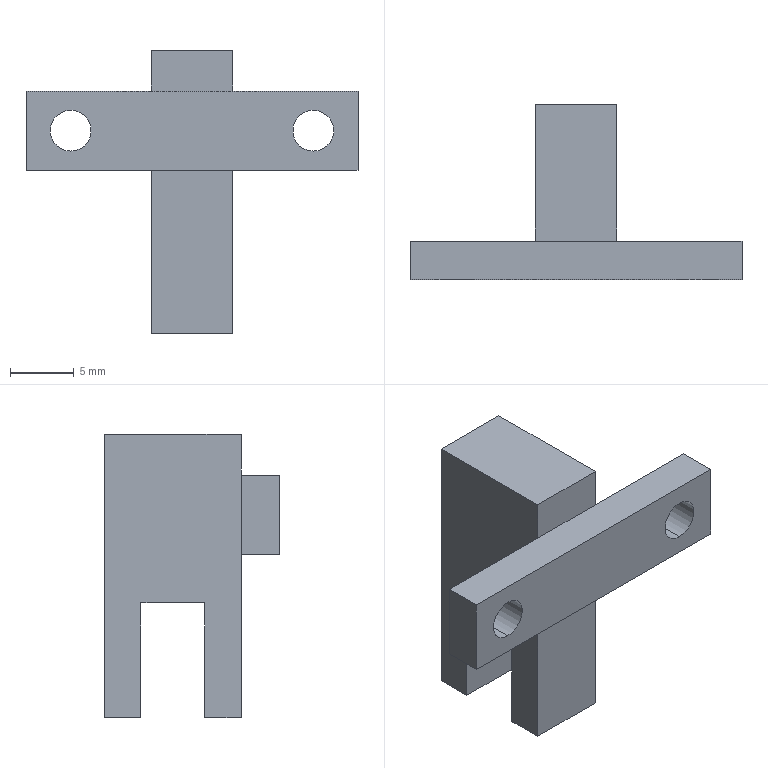Part | SolidWorks | features ICE 3, Extrusion 1 | 1 solid | 22 faces | box 26 x 13.7 x 22.2 mm | volume 1668 mm3 | plane 18 | cylinder 4 | commonest cylinder face diameters 3.2 x4
STEP:
#1=CARTESIAN_POINT('',(9.5,0.,-1.6));
#2=VERTEX_POINT('',#1);
#3=CARTESIAN_POINT('',(9.5,0.,1.6));
#4=VERTEX_POINT('',#3);
#5=CARTESIAN_POINT('',(9.5,0.,0.));
#6=DIRECTION('',(0.,1.,0.));
#7=DIRECTION('',(0.,0.,1.));
#8=AXIS2_PLACEMENT_3D('',#5,#6,#7);
#9=CIRCLE('',#8,1.6);
#10=EDGE_CURVE('',#2,#4,#9,.T.);
#11=ORIENTED_EDGE('',*,*,#10,.F.);
#12=CARTESIAN_POINT('',(9.5,3.,-1.6));
#13=VERTEX_POINT('',#12);
#14=CARTESIAN_POINT('',(9.5,-7.7,-1.6));
#15=DIRECTION('',(0.,1.,0.));
#16=VECTOR('',#15,1000.);
#17=LINE('',#14,#16);
#18=EDGE_CURVE('',#2,#13,#17,.T.);
#19=ORIENTED_EDGE('',*,*,#18,.T.);
#20=CARTESIAN_POINT('',(9.5,3.,1.6));
#21=VERTEX_POINT('',#20);
#22=CARTESIAN_POINT('',(9.5,3.,0.));
#23=DIRECTION('',(0.,1.,0.));
#24=DIRECTION('',(0.,0.,1.));
#25=AXIS2_PLACEMENT_3D('',#22,#23,#24);
#26=CIRCLE('',#25,1.6);
#27=EDGE_CURVE('',#13,#21,#26,.T.);
#28=ORIENTED_EDGE('',*,*,#27,.T.);
#29=CARTESIAN_POINT('',(9.5,-7.7,1.6));
#30=DIRECTION('',(0.,1.,0.));
#31=VECTOR('',#30,1000.);
#32=LINE('',#29,#31);
#33=EDGE_CURVE('',#4,#21,#32,.T.);
#34=ORIENTED_EDGE('',*,*,#33,.F.);
#35=EDGE_LOOP('',(#11,#19,#28,#34));
#36=FACE_OUTER_BOUND('',#35,.T.);
#37=CARTESIAN_POINT('',(9.5,-7.7,0.));
#38=DIRECTION('',(0.,1.,0.));
#39=DIRECTION('',(0.,0.,1.));
#40=AXIS2_PLACEMENT_3D('',#37,#38,#39);
#41=CYLINDRICAL_SURFACE('',#40,1.6);
#42=ADVANCED_FACE('',(#36),#41,.F.);
#43=CARTESIAN_POINT('',(-9.5,0.,-1.6));
#44=VERTEX_POINT('',#43);
#45=CARTESIAN_POINT('',(-9.5,0.,1.6));
#46=VERTEX_POINT('',#45);
#47=CARTESIAN_POINT('',(-9.5,0.,0.));
#48=DIRECTION('',(0.,1.,0.));
#49=DIRECTION('',(0.,0.,1.));
#50=AXIS2_PLACEMENT_3D('',#47,#48,#49);
#51=CIRCLE('',#50,1.6);
#52=EDGE_CURVE('',#44,#46,#51,.T.);
#53=ORIENTED_EDGE('',*,*,#52,.F.);
#54=CARTESIAN_POINT('',(-9.5,3.,-1.6));
#55=VERTEX_POINT('',#54);
#56=CARTESIAN_POINT('',(-9.5,-7.7,-1.6));
#57=DIRECTION('',(0.,1.,0.));
#58=VECTOR('',#57,1000.);
#59=LINE('',#56,#58);
#60=EDGE_CURVE('',#44,#55,#59,.T.);
#61=ORIENTED_EDGE('',*,*,#60,.T.);
#62=CARTESIAN_POINT('',(-9.5,3.,1.6));
#63=VERTEX_POINT('',#62);
#64=CARTESIAN_POINT('',(-9.5,3.,0.));
#65=DIRECTION('',(0.,1.,0.));
#66=DIRECTION('',(0.,0.,1.));
#67=AXIS2_PLACEMENT_3D('',#64,#65,#66);
#68=CIRCLE('',#67,1.6);
#69=EDGE_CURVE('',#55,#63,#68,.T.);
#70=ORIENTED_EDGE('',*,*,#69,.T.);
#71=CARTESIAN_POINT('',(-9.5,-7.7,1.6));
#72=DIRECTION('',(0.,1.,0.));
#73=VECTOR('',#72,1000.);
#74=LINE('',#71,#73);
#75=EDGE_CURVE('',#46,#63,#74,.T.);
#76=ORIENTED_EDGE('',*,*,#75,.F.);
#77=EDGE_LOOP('',(#53,#61,#70,#76));
#78=FACE_OUTER_BOUND('',#77,.T.);
#79=CARTESIAN_POINT('',(-9.5,-7.7,0.));
#80=DIRECTION('',(0.,1.,0.));
#81=DIRECTION('',(0.,0.,1.));
#82=AXIS2_PLACEMENT_3D('',#79,#80,#81);
#83=CYLINDRICAL_SURFACE('',#82,1.6);
#84=ADVANCED_FACE('',(#78),#83,.F.);
#85=CARTESIAN_POINT('',(3.2,13.7,-15.9));
#86=VERTEX_POINT('',#85);
#87=CARTESIAN_POINT('',(3.2,10.85,-15.9));
#88=VERTEX_POINT('',#87);
#89=CARTESIAN_POINT('',(3.2,13.7,-15.9));
#90=DIRECTION('',(0.,-1.,0.));
#91=VECTOR('',#90,1000.);
#92=LINE('',#89,#91);
#93=EDGE_CURVE('',#86,#88,#92,.T.);
#94=ORIENTED_EDGE('',*,*,#93,.T.);
#95=CARTESIAN_POINT('',(-3.2,10.85,-15.9));
#96=VERTEX_POINT('',#95);
#97=CARTESIAN_POINT('',(-3.2,10.85,-15.9));
#98=DIRECTION('',(-1.,0.,0.));
#99=VECTOR('',#98,1000.);
#100=LINE('',#97,#99);
#101=EDGE_CURVE('',#88,#96,#100,.T.);
#102=ORIENTED_EDGE('',*,*,#101,.T.);
#103=CARTESIAN_POINT('',(-3.2,13.7,-15.9));
#104=VERTEX_POINT('',#103);
#105=CARTESIAN_POINT('',(-3.2,13.7,-15.9));
#106=DIRECTION('',(0.,-1.,0.));
#107=VECTOR('',#106,1000.);
#108=LINE('',#105,#107);
#109=EDGE_CURVE('',#104,#96,#108,.T.);
#110=ORIENTED_EDGE('',*,*,#109,.F.);
#111=CARTESIAN_POINT('',(-3.2,13.7,-15.9));
#112=DIRECTION('',(-1.,0.,0.));
#113=VECTOR('',#112,1000.);
#114=LINE('',#111,#113);
#115=EDGE_CURVE('',#86,#104,#114,.T.);
#116=ORIENTED_EDGE('',*,*,#115,.F.);
#117=EDGE_LOOP('',(#94,#102,#110,#116));
#118=FACE_OUTER_BOUND('',#117,.T.);
#119=CARTESIAN_POINT('',(-3.2,13.7,-15.9));
#120=DIRECTION('',(0.,0.,1.));
#121=DIRECTION('',(1.,0.,0.));
#122=AXIS2_PLACEMENT_3D('',#119,#120,#121);
#123=PLANE('',#122);
#124=ADVANCED_FACE('',(#118),#123,.F.);
#125=CARTESIAN_POINT('',(-9.5,3.,0.));
#126=DIRECTION('',(0.,1.,0.));
#127=DIRECTION('',(0.,0.,1.));
#128=AXIS2_PLACEMENT_3D('',#125,#126,#127);
#129=CIRCLE('',#128,1.6);
#130=EDGE_CURVE('',#63,#55,#129,.T.);
#131=ORIENTED_EDGE('',*,*,#130,.F.);
#132=ORIENTED_EDGE('',*,*,#69,.F.);
#133=EDGE_LOOP('',(#131,#132));
#134=FACE_BOUND('',#133,.T.);
#135=CARTESIAN_POINT('',(-3.2,3.,-3.1));
#136=VERTEX_POINT('',#135);
#137=CARTESIAN_POINT('',(-3.2,3.,3.1));
#138=VERTEX_POINT('',#137);
#139=CARTESIAN_POINT('',(-3.2,3.,-15.9));
#140=DIRECTION('',(0.,0.,1.));
#141=VECTOR('',#140,1000.);
#142=LINE('',#139,#141);
#143=EDGE_CURVE('',#136,#138,#142,.T.);
#144=ORIENTED_EDGE('',*,*,#143,.F.);
#145=CARTESIAN_POINT('',(-13.,3.,-3.1));
#146=VERTEX_POINT('',#145);
#147=CARTESIAN_POINT('',(-13.,3.,-3.1));
#148=DIRECTION('',(-1.,0.,0.));
#149=VECTOR('',#148,1000.);
#150=LINE('',#147,#149);
#151=EDGE_CURVE('',#136,#146,#150,.T.);
#152=ORIENTED_EDGE('',*,*,#151,.T.);
#153=CARTESIAN_POINT('',(-13.,3.,3.1));
#154=VERTEX_POINT('',#153);
#155=CARTESIAN_POINT('',(-13.,3.,-3.1));
#156=DIRECTION('',(0.,0.,1.));
#157=VECTOR('',#156,1000.);
#158=LINE('',#155,#157);
#159=EDGE_CURVE('',#146,#154,#158,.T.);
#160=ORIENTED_EDGE('',*,*,#159,.T.);
#161=CARTESIAN_POINT('',(-13.,3.,3.1));
#162=DIRECTION('',(1.,0.,0.));
#163=VECTOR('',#162,1000.);
#164=LINE('',#161,#163);
#165=EDGE_CURVE('',#154,#138,#164,.T.);
#166=ORIENTED_EDGE('',*,*,#165,.T.);
#167=EDGE_LOOP('',(#144,#152,#160,#166));
#168=FACE_OUTER_BOUND('',#167,.T.);
#169=CARTESIAN_POINT('',(0.,3.,0.));
#170=DIRECTION('',(0.,1.,0.));
#171=DIRECTION('',(0.,0.,1.));
#172=AXIS2_PLACEMENT_3D('',#169,#170,#171);
#173=PLANE('',#172);
#174=ADVANCED_FACE('',(#134,#168),#173,.T.);
#175=CARTESIAN_POINT('',(13.,0.,3.1));
#176=VERTEX_POINT('',#175);
#177=CARTESIAN_POINT('',(13.,0.,-3.1));
#178=VERTEX_POINT('',#177);
#179=CARTESIAN_POINT('',(13.,0.,-3.1));
#180=DIRECTION('',(0.,0.,-1.));
#181=VECTOR('',#180,1000.);
#182=LINE('',#179,#181);
#183=EDGE_CURVE('',#176,#178,#182,.T.);
#184=ORIENTED_EDGE('',*,*,#183,.T.);
#185=CARTESIAN_POINT('',(13.,3.,-3.1));
#186=VERTEX_POINT('',#185);
#187=CARTESIAN_POINT('',(13.,3.,-3.1));
#188=DIRECTION('',(0.,-1.,0.));
#189=VECTOR('',#188,1000.);
#190=LINE('',#187,#189);
#191=EDGE_CURVE('',#186,#178,#190,.T.);
#192=ORIENTED_EDGE('',*,*,#191,.F.);
#193=CARTESIAN_POINT('',(13.,3.,3.1));
#194=VERTEX_POINT('',#193);
#195=CARTESIAN_POINT('',(13.,3.,-3.1));
#196=DIRECTION('',(0.,0.,-1.));
#197=VECTOR('',#196,1000.);
#198=LINE('',#195,#197);
#199=EDGE_CURVE('',#194,#186,#198,.T.);
#200=ORIENTED_EDGE('',*,*,#199,.F.);
#201=CARTESIAN_POINT('',(13.,3.,3.1));
#202=DIRECTION('',(0.,-1.,0.));
#203=VECTOR('',#202,1000.);
#204=LINE('',#201,#203);
#205=EDGE_CURVE('',#194,#176,#204,.T.);
#206=ORIENTED_EDGE('',*,*,#205,.T.);
#207=EDGE_LOOP('',(#184,#192,#200,#206));
#208=FACE_OUTER_BOUND('',#207,.T.);
#209=CARTESIAN_POINT('',(13.,3.,-3.1));
#210=DIRECTION('',(-1.,0.,0.));
#211=DIRECTION('',(0.,0.,1.));
#212=AXIS2_PLACEMENT_3D('',#209,#210,#211);
#213=PLANE('',#212);
#214=ADVANCED_FACE('',(#208),#213,.F.);
#215=CARTESIAN_POINT('',(-13.,0.,-3.1));
#216=VERTEX_POINT('',#215);
#217=CARTESIAN_POINT('',(-13.,0.,-3.1));
#218=DIRECTION('',(-1.,0.,0.));
#219=VECTOR('',#218,1000.);
#220=LINE('',#217,#219);
#221=EDGE_CURVE('',#178,#216,#220,.T.);
#222=ORIENTED_EDGE('',*,*,#221,.T.);
#223=CARTESIAN_POINT('',(-13.,3.,-3.1));
#224=DIRECTION('',(0.,-1.,0.));
#225=VECTOR('',#224,1000.);
#226=LINE('',#223,#225);
#227=EDGE_CURVE('',#146,#216,#226,.T.);
#228=ORIENTED_EDGE('',*,*,#227,.F.);
#229=ORIENTED_EDGE('',*,*,#151,.F.);
#230=CARTESIAN_POINT('',(3.2,3.,-3.1));
#231=VERTEX_POINT('',#230);
#232=CARTESIAN_POINT('',(-13.,3.,-3.1));
#233=DIRECTION('',(-1.,0.,0.));
#234=VECTOR('',#233,1000.);
#235=LINE('',#232,#234);
#236=EDGE_CURVE('',#231,#136,#235,.T.);
#237=ORIENTED_EDGE('',*,*,#236,.F.);
#238=CARTESIAN_POINT('',(-13.,3.,-3.1));
#239=DIRECTION('',(-1.,0.,0.));
#240=VECTOR('',#239,1000.);
#241=LINE('',#238,#240);
#242=EDGE_CURVE('',#186,#231,#241,.T.);
#243=ORIENTED_EDGE('',*,*,#242,.F.);
#244=ORIENTED_EDGE('',*,*,#191,.T.);
#245=EDGE_LOOP('',(#222,#228,#229,#237,#243,#244));
#246=FACE_OUTER_BOUND('',#245,.T.);
#247=CARTESIAN_POINT('',(-13.,3.,-3.1));
#248=DIRECTION('',(0.,0.,1.));
#249=DIRECTION('',(1.,0.,0.));
#250=AXIS2_PLACEMENT_3D('',#247,#248,#249);
#251=PLANE('',#250);
#252=ADVANCED_FACE('',(#246),#251,.F.);
#253=CARTESIAN_POINT('',(-13.,0.,3.1));
#254=VERTEX_POINT('',#253);
#255=CARTESIAN_POINT('',(-13.,0.,-3.1));
#256=DIRECTION('',(0.,0.,1.));
#257=VECTOR('',#256,1000.);
#258=LINE('',#255,#257);
#259=EDGE_CURVE('',#216,#254,#258,.T.);
#260=ORIENTED_EDGE('',*,*,#259,.T.);
#261=CARTESIAN_POINT('',(-13.,3.,3.1));
#262=DIRECTION('',(0.,-1.,0.));
#263=VECTOR('',#262,1000.);
#264=LINE('',#261,#263);
#265=EDGE_CURVE('',#154,#254,#264,.T.);
#266=ORIENTED_EDGE('',*,*,#265,.F.);
#267=ORIENTED_EDGE('',*,*,#159,.F.);
#268=ORIENTED_EDGE('',*,*,#227,.T.);
#269=EDGE_LOOP('',(#260,#266,#267,#268));
#270=FACE_OUTER_BOUND('',#269,.T.);
#271=CARTESIAN_POINT('',(-13.,3.,-3.1));
#272=DIRECTION('',(1.,0.,0.));
#273=DIRECTION('',(0.,0.,-1.));
#274=AXIS2_PLACEMENT_3D('',#271,#272,#273);
#275=PLANE('',#274);
#276=ADVANCED_FACE('',(#270),#275,.F.);
#277=CARTESIAN_POINT('',(-13.,0.,3.1));
#278=DIRECTION('',(1.,0.,0.));
#279=VECTOR('',#278,1000.);
#280=LINE('',#277,#279);
#281=EDGE_CURVE('',#254,#176,#280,.T.);
#282=ORIENTED_EDGE('',*,*,#281,.T.);
#283=ORIENTED_EDGE('',*,*,#205,.F.);
#284=CARTESIAN_POINT('',(3.2,3.,3.1));
#285=VERTEX_POINT('',#284);
#286=CARTESIAN_POINT('',(-13.,3.,3.1));
#287=DIRECTION('',(1.,0.,0.));
#288=VECTOR('',#287,1000.);
#289=LINE('',#286,#288);
#290=EDGE_CURVE('',#285,#194,#289,.T.);
#291=ORIENTED_EDGE('',*,*,#290,.F.);
#292=CARTESIAN_POINT('',(-13.,3.,3.1));
#293=DIRECTION('',(1.,0.,0.));
#294=VECTOR('',#293,1000.);
#295=LINE('',#292,#294);
#296=EDGE_CURVE('',#138,#285,#295,.T.);
#297=ORIENTED_EDGE('',*,*,#296,.F.);
#298=ORIENTED_EDGE('',*,*,#165,.F.);
#299=ORIENTED_EDGE('',*,*,#265,.T.);
#300=EDGE_LOOP('',(#282,#283,#291,#297,#298,#299));
#301=FACE_OUTER_BOUND('',#300,.T.);
#302=CARTESIAN_POINT('',(-13.,3.,3.1));
#303=DIRECTION('',(0.,0.,-1.));
#304=DIRECTION('',(-1.,0.,0.));
#305=AXIS2_PLACEMENT_3D('',#302,#303,#304);
#306=PLANE('',#305);
#307=ADVANCED_FACE('',(#301),#306,.F.);
#308=CARTESIAN_POINT('',(9.5,3.,0.));
#309=DIRECTION('',(0.,1.,0.));
#310=DIRECTION('',(0.,0.,1.));
#311=AXIS2_PLACEMENT_3D('',#308,#309,#310);
#312=CIRCLE('',#311,1.6);
#313=EDGE_CURVE('',#21,#13,#312,.T.);
#314=ORIENTED_EDGE('',*,*,#313,.F.);
#315=ORIENTED_EDGE('',*,*,#27,.F.);
#316=EDGE_LOOP('',(#314,#315));
#317=FACE_BOUND('',#316,.T.);
#318=CARTESIAN_POINT('',(3.2,3.,-15.9));
#319=DIRECTION('',(0.,0.,-1.));
#320=VECTOR('',#319,1000.);
#321=LINE('',#318,#320);
#322=EDGE_CURVE('',#285,#231,#321,.T.);
#323=ORIENTED_EDGE('',*,*,#322,.F.);
#324=ORIENTED_EDGE('',*,*,#290,.T.);
#325=ORIENTED_EDGE('',*,*,#199,.T.);
#326=ORIENTED_EDGE('',*,*,#242,.T.);
#327=EDGE_LOOP('',(#323,#324,#325,#326));
#328=FACE_OUTER_BOUND('',#327,.T.);
#329=CARTESIAN_POINT('',(0.,3.,0.));
#330=DIRECTION('',(0.,1.,0.));
#331=DIRECTION('',(0.,0.,1.));
#332=AXIS2_PLACEMENT_3D('',#329,#330,#331);
#333=PLANE('',#332);
#334=ADVANCED_FACE('',(#317,#328),#333,.T.);
#335=CARTESIAN_POINT('',(9.5,0.,0.));
#336=DIRECTION('',(0.,1.,0.));
#337=DIRECTION('',(0.,0.,1.));
#338=AXIS2_PLACEMENT_3D('',#335,#336,#337);
#339=CIRCLE('',#338,1.6);
#340=EDGE_CURVE('',#4,#2,#339,.T.);
#341=ORIENTED_EDGE('',*,*,#340,.T.);
#342=ORIENTED_EDGE('',*,*,#10,.T.);
#343=EDGE_LOOP('',(#341,#342));
#344=FACE_BOUND('',#343,.T.);
#345=CARTESIAN_POINT('',(-9.5,0.,0.));
#346=DIRECTION('',(0.,1.,0.));
#347=DIRECTION('',(0.,0.,1.));
#348=AXIS2_PLACEMENT_3D('',#345,#346,#347);
#349=CIRCLE('',#348,1.6);
#350=EDGE_CURVE('',#46,#44,#349,.T.);
#351=ORIENTED_EDGE('',*,*,#350,.T.);
#352=ORIENTED_EDGE('',*,*,#52,.T.);
#353=EDGE_LOOP('',(#351,#352));
#354=FACE_BOUND('',#353,.T.);
#355=ORIENTED_EDGE('',*,*,#183,.F.);
#356=ORIENTED_EDGE('',*,*,#281,.F.);
#357=ORIENTED_EDGE('',*,*,#259,.F.);
#358=ORIENTED_EDGE('',*,*,#221,.F.);
#359=EDGE_LOOP('',(#355,#356,#357,#358));
#360=FACE_OUTER_BOUND('',#359,.T.);
#361=CARTESIAN_POINT('',(0.,0.,0.));
#362=DIRECTION('',(0.,1.,0.));
#363=DIRECTION('',(0.,0.,1.));
#364=AXIS2_PLACEMENT_3D('',#361,#362,#363);
#365=PLANE('',#364);
#366=ADVANCED_FACE('',(#344,#354,#360),#365,.F.);
#367=CARTESIAN_POINT('',(3.2,3.,-15.9));
#368=VERTEX_POINT('',#367);
#369=CARTESIAN_POINT('',(3.2,3.,-15.9));
#370=DIRECTION('',(0.,0.,-1.));
#371=VECTOR('',#370,1000.);
#372=LINE('',#369,#371);
#373=EDGE_CURVE('',#231,#368,#372,.T.);
#374=ORIENTED_EDGE('',*,*,#373,.F.);
#375=ORIENTED_EDGE('',*,*,#236,.T.);
#376=CARTESIAN_POINT('',(-3.2,3.,-15.9));
#377=VERTEX_POINT('',#376);
#378=CARTESIAN_POINT('',(-3.2,3.,-15.9));
#379=DIRECTION('',(0.,0.,1.));
#380=VECTOR('',#379,1000.);
#381=LINE('',#378,#380);
#382=EDGE_CURVE('',#377,#136,#381,.T.);
#383=ORIENTED_EDGE('',*,*,#382,.F.);
#384=CARTESIAN_POINT('',(-3.2,3.,-15.9));
#385=DIRECTION('',(-1.,0.,0.));
#386=VECTOR('',#385,1000.);
#387=LINE('',#384,#386);
#388=EDGE_CURVE('',#368,#377,#387,.T.);
#389=ORIENTED_EDGE('',*,*,#388,.F.);
#390=EDGE_LOOP('',(#374,#375,#383,#389));
#391=FACE_OUTER_BOUND('',#390,.T.);
#392=CARTESIAN_POINT('',(0.,3.,0.));
#393=DIRECTION('',(0.,1.,0.));
#394=DIRECTION('',(0.,0.,1.));
#395=AXIS2_PLACEMENT_3D('',#392,#393,#394);
#396=PLANE('',#395);
#397=ADVANCED_FACE('',(#391),#396,.F.);
#398=CARTESIAN_POINT('',(-3.2,3.,6.3));
#399=VERTEX_POINT('',#398);
#400=CARTESIAN_POINT('',(-3.2,3.,-15.9));
#401=DIRECTION('',(0.,0.,1.));
#402=VECTOR('',#401,1000.);
#403=LINE('',#400,#402);
#404=EDGE_CURVE('',#138,#399,#403,.T.);
#405=ORIENTED_EDGE('',*,*,#404,.F.);
#406=ORIENTED_EDGE('',*,*,#296,.T.);
#407=CARTESIAN_POINT('',(3.2,3.,6.3));
#408=VERTEX_POINT('',#407);
#409=CARTESIAN_POINT('',(3.2,3.,-15.9));
#410=DIRECTION('',(0.,0.,-1.));
#411=VECTOR('',#410,1000.);
#412=LINE('',#409,#411);
#413=EDGE_CURVE('',#408,#285,#412,.T.);
#414=ORIENTED_EDGE('',*,*,#413,.F.);
#415=CARTESIAN_POINT('',(-3.2,3.,6.3));
#416=DIRECTION('',(1.,0.,0.));
#417=VECTOR('',#416,1000.);
#418=LINE('',#415,#417);
#419=EDGE_CURVE('',#399,#408,#418,.T.);
#420=ORIENTED_EDGE('',*,*,#419,.F.);
#421=EDGE_LOOP('',(#405,#406,#414,#420));
#422=FACE_OUTER_BOUND('',#421,.T.);
#423=CARTESIAN_POINT('',(0.,3.,0.));
#424=DIRECTION('',(0.,1.,0.));
#425=DIRECTION('',(0.,0.,1.));
#426=AXIS2_PLACEMENT_3D('',#423,#424,#425);
#427=PLANE('',#426);
#428=ADVANCED_FACE('',(#422),#427,.F.);
#429=ORIENTED_EDGE('',*,*,#109,.T.);
#430=CARTESIAN_POINT('',(-3.2,10.85,-6.9));
#431=VERTEX_POINT('',#430);
#432=CARTESIAN_POINT('',(-3.2,10.85,-15.9));
#433=DIRECTION('',(0.,0.,-1.));
#434=VECTOR('',#433,1000.);
#435=LINE('',#432,#434);
#436=EDGE_CURVE('',#431,#96,#435,.T.);
#437=ORIENTED_EDGE('',*,*,#436,.F.);
#438=CARTESIAN_POINT('',(-3.2,5.85,-6.9));
#439=VERTEX_POINT('',#438);
#440=CARTESIAN_POINT('',(-3.2,10.85,-6.9));
#441=DIRECTION('',(0.,1.,0.));
#442=VECTOR('',#441,1000.);
#443=LINE('',#440,#442);
#444=EDGE_CURVE('',#439,#431,#443,.T.);
#445=ORIENTED_EDGE('',*,*,#444,.F.);
#446=CARTESIAN_POINT('',(-3.2,5.85,-15.9));
#447=VERTEX_POINT('',#446);
#448=CARTESIAN_POINT('',(-3.2,5.85,-15.9));
#449=DIRECTION('',(0.,0.,1.));
#450=VECTOR('',#449,1000.);
#451=LINE('',#448,#450);
#452=EDGE_CURVE('',#447,#439,#451,.T.);
#453=ORIENTED_EDGE('',*,*,#452,.F.);
#454=CARTESIAN_POINT('',(-3.2,13.7,-15.9));
#455=DIRECTION('',(0.,-1.,0.));
#456=VECTOR('',#455,1000.);
#457=LINE('',#454,#456);
#458=EDGE_CURVE('',#447,#377,#457,.T.);
#459=ORIENTED_EDGE('',*,*,#458,.T.);
#460=ORIENTED_EDGE('',*,*,#382,.T.);
#461=ORIENTED_EDGE('',*,*,#143,.T.);
#462=ORIENTED_EDGE('',*,*,#404,.T.);
#463=CARTESIAN_POINT('',(-3.2,13.7,6.3));
#464=VERTEX_POINT('',#463);
#465=CARTESIAN_POINT('',(-3.2,13.7,6.3));
#466=DIRECTION('',(0.,-1.,0.));
#467=VECTOR('',#466,1000.);
#468=LINE('',#465,#467);
#469=EDGE_CURVE('',#464,#399,#468,.T.);
#470=ORIENTED_EDGE('',*,*,#469,.F.);
#471=CARTESIAN_POINT('',(-3.2,13.7,-15.9));
#472=DIRECTION('',(0.,0.,1.));
#473=VECTOR('',#472,1000.);
#474=LINE('',#471,#473);
#475=EDGE_CURVE('',#104,#464,#474,.T.);
#476=ORIENTED_EDGE('',*,*,#475,.F.);
#477=EDGE_LOOP('',(#429,#437,#445,#453,#459,#460,#461,#462,#470,#476));
#478=FACE_OUTER_BOUND('',#477,.T.);
#479=CARTESIAN_POINT('',(-3.2,13.7,-15.9));
#480=DIRECTION('',(1.,0.,0.));
#481=DIRECTION('',(0.,0.,-1.));
#482=AXIS2_PLACEMENT_3D('',#479,#480,#481);
#483=PLANE('',#482);
#484=ADVANCED_FACE('',(#478),#483,.F.);
#485=ORIENTED_EDGE('',*,*,#419,.T.);
#486=CARTESIAN_POINT('',(3.2,13.7,6.3));
#487=VERTEX_POINT('',#486);
#488=CARTESIAN_POINT('',(3.2,13.7,6.3));
#489=DIRECTION('',(0.,-1.,0.));
#490=VECTOR('',#489,1000.);
#491=LINE('',#488,#490);
#492=EDGE_CURVE('',#487,#408,#491,.T.);
#493=ORIENTED_EDGE('',*,*,#492,.F.);
#494=CARTESIAN_POINT('',(-3.2,13.7,6.3));
#495=DIRECTION('',(1.,0.,0.));
#496=VECTOR('',#495,1000.);
#497=LINE('',#494,#496);
#498=EDGE_CURVE('',#464,#487,#497,.T.);
#499=ORIENTED_EDGE('',*,*,#498,.F.);
#500=ORIENTED_EDGE('',*,*,#469,.T.);
#501=EDGE_LOOP('',(#485,#493,#499,#500));
#502=FACE_OUTER_BOUND('',#501,.T.);
#503=CARTESIAN_POINT('',(-3.2,13.7,6.3));
#504=DIRECTION('',(0.,0.,-1.));
#505=DIRECTION('',(-1.,0.,0.));
#506=AXIS2_PLACEMENT_3D('',#503,#504,#505);
#507=PLANE('',#506);
#508=ADVANCED_FACE('',(#502),#507,.F.);
#509=CARTESIAN_POINT('',(3.2,5.85,-6.9));
#510=VERTEX_POINT('',#509);
#511=CARTESIAN_POINT('',(3.2,10.85,-6.9));
#512=VERTEX_POINT('',#511);
#513=CARTESIAN_POINT('',(3.2,13.7,-6.9));
#514=DIRECTION('',(0.,1.,0.));
#515=VECTOR('',#514,1000.);
#516=LINE('',#513,#515);
#517=EDGE_CURVE('',#510,#512,#516,.T.);
#518=ORIENTED_EDGE('',*,*,#517,.T.);
#519=CARTESIAN_POINT('',(3.2,10.85,-15.9));
#520=DIRECTION('',(0.,0.,-1.));
#521=VECTOR('',#520,1000.);
#522=LINE('',#519,#521);
#523=EDGE_CURVE('',#512,#88,#522,.T.);
#524=ORIENTED_EDGE('',*,*,#523,.T.);
#525=ORIENTED_EDGE('',*,*,#93,.F.);
#526=CARTESIAN_POINT('',(3.2,13.7,-15.9));
#527=DIRECTION('',(0.,0.,-1.));
#528=VECTOR('',#527,1000.);
#529=LINE('',#526,#528);
#530=EDGE_CURVE('',#487,#86,#529,.T.);
#531=ORIENTED_EDGE('',*,*,#530,.F.);
#532=ORIENTED_EDGE('',*,*,#492,.T.);
#533=ORIENTED_EDGE('',*,*,#413,.T.);
#534=ORIENTED_EDGE('',*,*,#322,.T.);
#535=ORIENTED_EDGE('',*,*,#373,.T.);
#536=CARTESIAN_POINT('',(3.2,5.85,-15.9));
#537=VERTEX_POINT('',#536);
#538=CARTESIAN_POINT('',(3.2,13.7,-15.9));
#539=DIRECTION('',(0.,-1.,0.));
#540=VECTOR('',#539,1000.);
#541=LINE('',#538,#540);
#542=EDGE_CURVE('',#537,#368,#541,.T.);
#543=ORIENTED_EDGE('',*,*,#542,.F.);
#544=CARTESIAN_POINT('',(3.2,5.85,-15.9));
#545=DIRECTION('',(0.,0.,1.));
#546=VECTOR('',#545,1000.);
#547=LINE('',#544,#546);
#548=EDGE_CURVE('',#537,#510,#547,.T.);
#549=ORIENTED_EDGE('',*,*,#548,.T.);
#550=EDGE_LOOP('',(#518,#524,#525,#531,#532,#533,#534,#535,#543,#549));
#551=FACE_OUTER_BOUND('',#550,.T.);
#552=CARTESIAN_POINT('',(3.2,13.7,-15.9));
#553=DIRECTION('',(-1.,0.,0.));
#554=DIRECTION('',(0.,0.,1.));
#555=AXIS2_PLACEMENT_3D('',#552,#553,#554);
#556=PLANE('',#555);
#557=ADVANCED_FACE('',(#551),#556,.F.);
#558=ORIENTED_EDGE('',*,*,#458,.F.);
#559=CARTESIAN_POINT('',(-3.2,5.85,-15.9));
#560=DIRECTION('',(1.,0.,0.));
#561=VECTOR('',#560,1000.);
#562=LINE('',#559,#561);
#563=EDGE_CURVE('',#447,#537,#562,.T.);
#564=ORIENTED_EDGE('',*,*,#563,.T.);
#565=ORIENTED_EDGE('',*,*,#542,.T.);
#566=ORIENTED_EDGE('',*,*,#388,.T.);
#567=EDGE_LOOP('',(#558,#564,#565,#566));
#568=FACE_OUTER_BOUND('',#567,.T.);
#569=CARTESIAN_POINT('',(-3.2,13.7,-15.9));
#570=DIRECTION('',(0.,0.,1.));
#571=DIRECTION('',(1.,0.,0.));
#572=AXIS2_PLACEMENT_3D('',#569,#570,#571);
#573=PLANE('',#572);
#574=ADVANCED_FACE('',(#568),#573,.F.);
#575=ORIENTED_EDGE('',*,*,#475,.T.);
#576=ORIENTED_EDGE('',*,*,#498,.T.);
#577=ORIENTED_EDGE('',*,*,#530,.T.);
#578=ORIENTED_EDGE('',*,*,#115,.T.);
#579=EDGE_LOOP('',(#575,#576,#577,#578));
#580=FACE_OUTER_BOUND('',#579,.T.);
#581=CARTESIAN_POINT('',(0.,13.7,0.));
#582=DIRECTION('',(0.,1.,0.));
#583=DIRECTION('',(0.,0.,1.));
#584=AXIS2_PLACEMENT_3D('',#581,#582,#583);
#585=PLANE('',#584);
#586=ADVANCED_FACE('',(#580),#585,.T.);
#587=CARTESIAN_POINT('',(7.5,5.85,-6.9));
#588=DIRECTION('',(-1.,0.,0.));
#589=VECTOR('',#588,1000.);
#590=LINE('',#587,#589);
#591=EDGE_CURVE('',#510,#439,#590,.T.);
#592=ORIENTED_EDGE('',*,*,#591,.T.);
#593=ORIENTED_EDGE('',*,*,#444,.T.);
#594=CARTESIAN_POINT('',(7.5,10.85,-6.9));
#595=DIRECTION('',(-1.,0.,0.));
#596=VECTOR('',#595,1000.);
#597=LINE('',#594,#596);
#598=EDGE_CURVE('',#512,#431,#597,.T.);
#599=ORIENTED_EDGE('',*,*,#598,.F.);
#600=ORIENTED_EDGE('',*,*,#517,.F.);
#601=EDGE_LOOP('',(#592,#593,#599,#600));
#602=FACE_OUTER_BOUND('',#601,.T.);
#603=CARTESIAN_POINT('',(7.5,10.85,-6.9));
#604=DIRECTION('',(0.,0.,1.));
#605=DIRECTION('',(1.,0.,0.));
#606=AXIS2_PLACEMENT_3D('',#603,#604,#605);
#607=PLANE('',#606);
#608=ADVANCED_FACE('',(#602),#607,.F.);
#609=ORIENTED_EDGE('',*,*,#598,.T.);
#610=ORIENTED_EDGE('',*,*,#436,.T.);
#611=ORIENTED_EDGE('',*,*,#101,.F.);
#612=ORIENTED_EDGE('',*,*,#523,.F.);
#613=EDGE_LOOP('',(#609,#610,#611,#612));
#614=FACE_OUTER_BOUND('',#613,.T.);
#615=CARTESIAN_POINT('',(7.5,10.85,-15.9));
#616=DIRECTION('',(0.,1.,0.));
#617=DIRECTION('',(0.,0.,1.));
#618=AXIS2_PLACEMENT_3D('',#615,#616,#617);
#619=PLANE('',#618);
#620=ADVANCED_FACE('',(#614),#619,.F.);
#621=ORIENTED_EDGE('',*,*,#563,.F.);
#622=ORIENTED_EDGE('',*,*,#452,.T.);
#623=ORIENTED_EDGE('',*,*,#591,.F.);
#624=ORIENTED_EDGE('',*,*,#548,.F.);
#625=EDGE_LOOP('',(#621,#622,#623,#624));
#626=FACE_OUTER_BOUND('',#625,.T.);
#627=CARTESIAN_POINT('',(7.5,5.85,-15.9));
#628=DIRECTION('',(0.,-1.,0.));
#629=DIRECTION('',(0.,0.,-1.));
#630=AXIS2_PLACEMENT_3D('',#627,#628,#629);
#631=PLANE('',#630);
#632=ADVANCED_FACE('',(#626),#631,.F.);
#633=ORIENTED_EDGE('',*,*,#60,.F.);
#634=ORIENTED_EDGE('',*,*,#350,.F.);
#635=ORIENTED_EDGE('',*,*,#75,.T.);
#636=ORIENTED_EDGE('',*,*,#130,.T.);
#637=EDGE_LOOP('',(#633,#634,#635,#636));
#638=FACE_OUTER_BOUND('',#637,.T.);
#639=CARTESIAN_POINT('',(-9.5,-7.7,0.));
#640=DIRECTION('',(0.,1.,0.));
#641=DIRECTION('',(0.,0.,1.));
#642=AXIS2_PLACEMENT_3D('',#639,#640,#641);
#643=CYLINDRICAL_SURFACE('',#642,1.6);
#644=ADVANCED_FACE('',(#638),#643,.F.);
#645=ORIENTED_EDGE('',*,*,#18,.F.);
#646=ORIENTED_EDGE('',*,*,#340,.F.);
#647=ORIENTED_EDGE('',*,*,#33,.T.);
#648=ORIENTED_EDGE('',*,*,#313,.T.);
#649=EDGE_LOOP('',(#645,#646,#647,#648));
#650=FACE_OUTER_BOUND('',#649,.T.);
#651=CARTESIAN_POINT('',(9.5,-7.7,0.));
#652=DIRECTION('',(0.,1.,0.));
#653=DIRECTION('',(0.,0.,1.));
#654=AXIS2_PLACEMENT_3D('',#651,#652,#653);
#655=CYLINDRICAL_SURFACE('',#654,1.6);
#656=ADVANCED_FACE('',(#650),#655,.F.);
#657=CLOSED_SHELL('',(#42,#84,#124,#174,#214,#252,#276,#307,#334,#366,#397,#428,#484,#508,#557,#574,#586,#608,#620,#632,#644,#656));
#658=MANIFOLD_SOLID_BREP('',#657);
#659=CARTESIAN_POINT('',(0.,0.,0.));
#660=DIRECTION('',(0.,0.,1.));
#661=DIRECTION('',(1.,0.,0.));
#662=AXIS2_PLACEMENT_3D('',#659,#660,#661);
#663=(LENGTH_UNIT()NAMED_UNIT(*)SI_UNIT(.MILLI.,.METRE.));
#664=UNCERTAINTY_MEASURE_WITH_UNIT(LENGTH_MEASURE(0.00001),#663,'','');
#665=(NAMED_UNIT(*)PLANE_ANGLE_UNIT()SI_UNIT($,.RADIAN.));
#666=(NAMED_UNIT(*)SI_UNIT($,.STERADIAN.)SOLID_ANGLE_UNIT());
#667=(GEOMETRIC_REPRESENTATION_CONTEXT(3)GLOBAL_UNCERTAINTY_ASSIGNED_CONTEXT((#664))GLOBAL_UNIT_ASSIGNED_CONTEXT((#663,#665,#666))REPRESENTATION_CONTEXT('',''));
#668=ADVANCED_BREP_SHAPE_REPRESENTATION('',(#658,#662),#667);